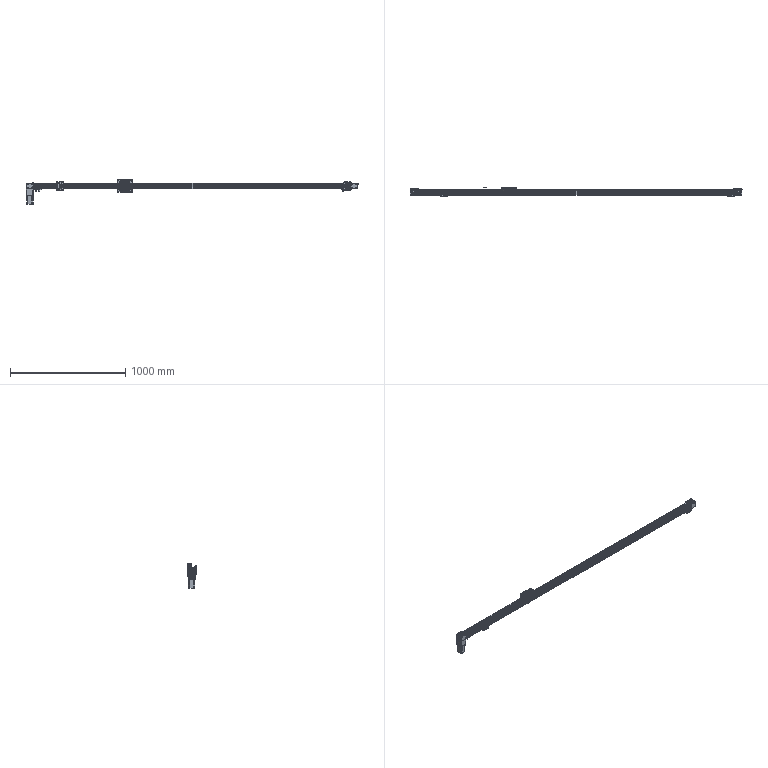Part | SolidWorks | features CompositeCurve 10 | 26 solids | 6077 faces | volume 6127819 mm3 | plane 3167 | cylinder 1811 | cone 714 | spline 241 | torus 128 | sphere 16 | commonest cylinder face diameters 0.2 x382 2 x125 0.4 x119 0.6 x105 5 x85 5.5 x82